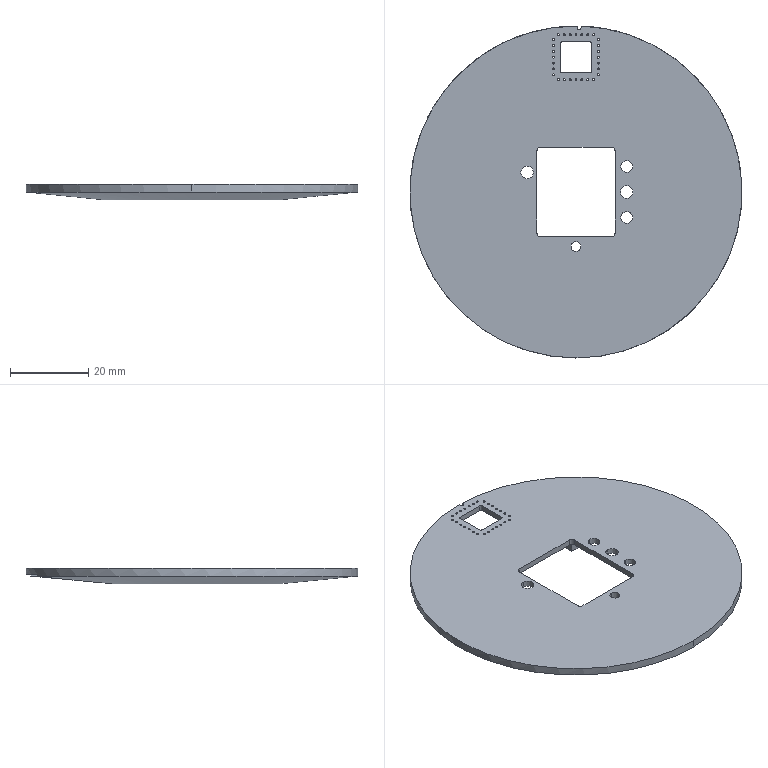CAM job | NX | 3-axis milling, drilling | part box 85 x 85 x 4 mm | stock box 89 x 89 x 5 mm
Tools:
number,name,description,diameter,corner_radius,flute_length,length,flutes
1,D6A45,Milling Tool-5 Parameters,6.0,0.0,50.0,75.0,2
22,2.5ZT,Drilling Tool,2.5,0.0,35.0,50.0,2
13,3.2ZT,Drilling Tool,3.2,0.0,35.0,50.0,2
24,0.5ZT,Drilling Tool,0.5,0.0,35.0,50.0,2
4,D10,Milling Tool-5 Parameters,10.0,0.0,50.0,75.0,2
14,D10JING,Milling Tool-5 Parameters,10.0,0.0,50.0,75.0,2
16,D6,Milling Tool-5 Parameters,6.0,0.0,50.0,75.0,2
17,D3,Milling Tool-5 Parameters,3.0,0.0,50.0,75.0,2
18,D2,Milling Tool-5 Parameters,2.0,0.0,50.0,75.0,2
19,D1,Milling Tool-5 Parameters,1.0,0.0,50.0,75.0,2
7,D4R0.5,Milling Tool-5 Parameters,4.0,0.5,50.0,75.0,2
Operations:
program,operation,operation_type,tool,method,geometry_group,spindle_rpm,surface_speed,feed_per_tooth,feed_cut,feed_plunge,cut_length_mm,path_length_mm,cut_time_min,machine_time_min
1AB胶-反面见光,FLOOR_WALL,VolumeBased25DMillingOperation,D10JING,METHOD,A,6500.0,1286.0,0.1154,1500.0,100.0,1284.997,1338.697,0.8567,0.862
1AB胶-反面见光,DRILLING,Operation,D6A45,METHOD,A,5000.0,94.0,0.025,250.0,0.0,132.0,588.748,0.528,0.5737
1AB胶-反面见光,DRILLING_COPY_COPY,Operation,2.5ZT,METHOD,A,2000.0,21.0,0.0375,150.0,0.0,9.251,78.502,0.0617,0.0686
1AB胶-反面见光,DRILLING_COPY,Operation,3.2ZT,METHOD,A,2000.0,21.0,0.0375,150.0,0.0,18.923,127.004,0.1262,0.137
1AB胶-反面见光,DRILLING_COPY_COPY_1,Operation,0.5ZT,METHOD,A,2000.0,3.0,0.0125,50.0,0.0,214.206,660.357,4.284,4.329
1AB胶-反面见光,ZLEVEL_PROFILE_1,ZLevelMilling,D10,METHOD,A,7500.0,235.0,0.2,3000.0,1000.0,1291.441,1351.841,0.4604,0.4665
1AB胶-反面见光,CAVITY_MILL,CavityMilling,D10,METHOD,A,7500.0,235.0,0.2,3000.0,1000.0,2467.522,2685.351,0.9388,0.9606
1AB胶-反面见光,CAVITY_MILL_1,CavityMilling,D6,METHOD,A,7500.0,141.0,0.12,1800.0,100.0,316.025,1204.207,0.1756,0.2644
1AB胶-反面见光,CAVITY_MILL_COPY_1,CavityMilling,D3,METHOD,A,7500.0,70.0,0.08,1200.0,100.0,508.558,1623.212,0.4238,0.5353
1AB胶-反面见光,FLOOR_WALL_1_COPY_COPY,VolumeBased25DMillingOperation,D3,METHOD,A,7500.0,235.0,0.08,1200.0,1000.0,2132.522,2771.082,1.788,1.852
1AB胶-反面见光,ZLEVEL_PROFILE,ZLevelMilling,D3,METHOD,A,7500.0,235.0,0.0667,1000.0,100.0,101.978,262.608,0.102,0.118
1AB胶-反面见光,CAVITY_MILL_COPY,CavityMilling,D2,METHOD,A,7500.0,47.0,0.0533,800.0,100.0,952.699,5008.975,1.191,1.597
1AB胶-反面见光,HOLE_MILLING,CylinderMilling,D2,METHOD,A,7500.0,47.0,0.0533,800.0,100.0,121.65,266.65,0.1521,0.1666
1AB胶-反面见光,CAVITY_MILL_COPY_COPY,CavityMilling,D1,METHOD,A,7500.0,47.0,0.0533,800.0,100.0,220.966,712.188,0.2762,0.3253
1AB胶-反面见光,ZLEVEL_PROFILE_1_COPY,ZLevelMilling,D1,METHOD,A,7500.0,23.0,0.0533,800.0,1000.0,1134.911,1266.14,1.404,1.417
1AB胶-反面见光,PLANAR_PROFILE,PlanarMilling,D1,METHOD,A,7500.0,23.0,0.0533,800.0,100.0,149.413,217.413,0.1868,0.1936
1AB胶-反面见光,ZLEVEL_PROFILE_1_1,ZLevelMilling,D4R0.5,METHOD,A,7500.0,94.0,0.1667,2500.0,1000.0,44522.86,44583.079,17.81,17.816
1AB胶-反面见光,PLANAR_MILL,PlanarMilling,D6A45,METHOD,A,7500.0,141.0,0.0833,1250.0,100.0,126.907,275.506,0.1015,0.1164
1AB胶-反面见光,PLANAR_MILL_COPY,PlanarMilling,D6A45,METHOD,A,7500.0,141.0,0.0833,1250.0,100.0,240.134,992.829,0.1921,0.2674
1AB胶-反面见光,刀补18,CylinderMilling,D2,METHOD,A,7500.0,47.0,0.0533,800.0,100.0,20.877,165.877,0.0261,0.0406
1AB胶-反面见光,ZLEVEL_PROFILE_1_COPY_1,ZLevelMilling,D6,METHOD,A,7500.0,141.0,0.08,1200.0,1000.0,1188.825,1251.625,0.9959,1.002